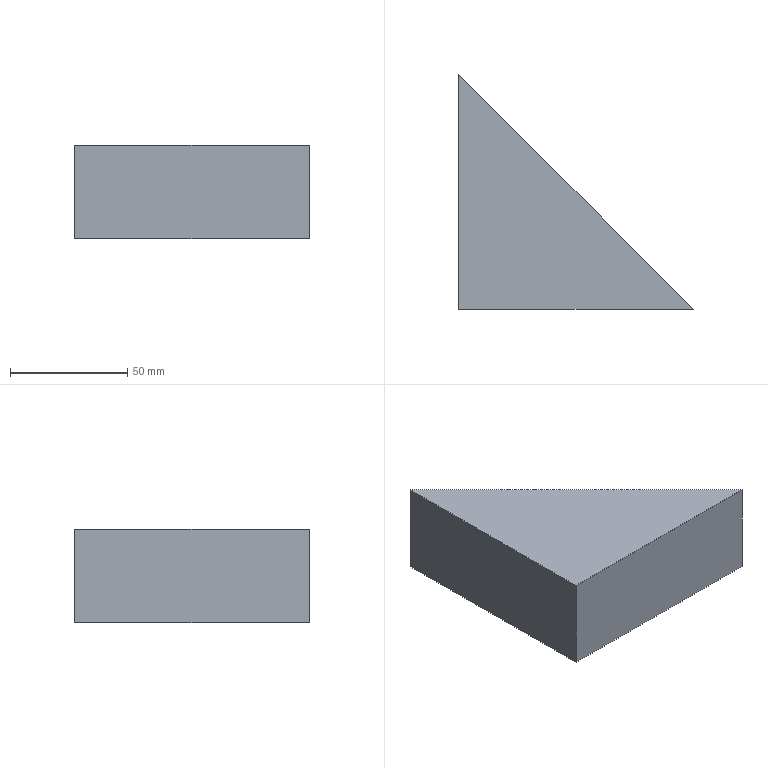Part | 1 solid | 9 faces | box 100 x 100 x 40 mm | volume 67460 mm3 | plane 9
STEP:
#1=CARTESIAN_POINT('',(3.,97.,35.));
#2=VERTEX_POINT('',#1);
#3=CARTESIAN_POINT('',(3.,97.,5.));
#4=VERTEX_POINT('',#3);
#5=CARTESIAN_POINT('',(3.,97.,40.));
#6=DIRECTION('',(0.,0.,-1.));
#7=VECTOR('',#6,1000.);
#8=LINE('',#5,#7);
#9=EDGE_CURVE('',#2,#4,#8,.T.);
#10=ORIENTED_EDGE('',*,*,#9,.T.);
#11=CARTESIAN_POINT('',(97.,3.,5.));
#12=VERTEX_POINT('',#11);
#13=CARTESIAN_POINT('',(100.,0.,5.));
#14=DIRECTION('',(0.7071,-0.7071,0.));
#15=VECTOR('',#14,1000.);
#16=LINE('',#13,#15);
#17=EDGE_CURVE('',#4,#12,#16,.T.);
#18=ORIENTED_EDGE('',*,*,#17,.T.);
#19=CARTESIAN_POINT('',(97.,3.,35.));
#20=VERTEX_POINT('',#19);
#21=CARTESIAN_POINT('',(97.,3.,40.));
#22=DIRECTION('',(0.,0.,1.));
#23=VECTOR('',#22,1000.);
#24=LINE('',#21,#23);
#25=EDGE_CURVE('',#12,#20,#24,.T.);
#26=ORIENTED_EDGE('',*,*,#25,.T.);
#27=CARTESIAN_POINT('',(100.,0.,35.));
#28=DIRECTION('',(0.7071,-0.7071,0.));
#29=VECTOR('',#28,1000.);
#30=LINE('',#27,#29);
#31=EDGE_CURVE('',#2,#20,#30,.T.);
#32=ORIENTED_EDGE('',*,*,#31,.F.);
#33=EDGE_LOOP('',(#10,#18,#26,#32));
#34=FACE_BOUND('',#33,.T.);
#35=CARTESIAN_POINT('',(100.,0.,0.));
#36=VERTEX_POINT('',#35);
#37=CARTESIAN_POINT('',(0.,100.,0.));
#38=VERTEX_POINT('',#37);
#39=CARTESIAN_POINT('',(100.,0.,0.));
#40=DIRECTION('',(-0.7071,0.7071,0.));
#41=VECTOR('',#40,1000.);
#42=LINE('',#39,#41);
#43=EDGE_CURVE('',#36,#38,#42,.T.);
#44=ORIENTED_EDGE('',*,*,#43,.T.);
#45=CARTESIAN_POINT('',(0.,100.,40.));
#46=VERTEX_POINT('',#45);
#47=CARTESIAN_POINT('',(0.,100.,40.));
#48=DIRECTION('',(0.,0.,-1.));
#49=VECTOR('',#48,1000.);
#50=LINE('',#47,#49);
#51=EDGE_CURVE('',#46,#38,#50,.T.);
#52=ORIENTED_EDGE('',*,*,#51,.F.);
#53=CARTESIAN_POINT('',(100.,0.,40.));
#54=VERTEX_POINT('',#53);
#55=CARTESIAN_POINT('',(100.,0.,40.));
#56=DIRECTION('',(-0.7071,0.7071,0.));
#57=VECTOR('',#56,1000.);
#58=LINE('',#55,#57);
#59=EDGE_CURVE('',#54,#46,#58,.T.);
#60=ORIENTED_EDGE('',*,*,#59,.F.);
#61=CARTESIAN_POINT('',(100.,0.,40.));
#62=DIRECTION('',(0.,0.,-1.));
#63=VECTOR('',#62,1000.);
#64=LINE('',#61,#63);
#65=EDGE_CURVE('',#54,#36,#64,.T.);
#66=ORIENTED_EDGE('',*,*,#65,.T.);
#67=EDGE_LOOP('',(#44,#52,#60,#66));
#68=FACE_OUTER_BOUND('',#67,.T.);
#69=CARTESIAN_POINT('',(100.,0.,40.));
#70=DIRECTION('',(-0.7071,-0.7071,0.));
#71=DIRECTION('',(0.7071,-0.7071,0.));
#72=AXIS2_PLACEMENT_3D('',#69,#70,#71);
#73=PLANE('',#72);
#74=ADVANCED_FACE('',(#34,#68),#73,.F.);
#75=CARTESIAN_POINT('',(0.,0.,0.));
#76=VERTEX_POINT('',#75);
#77=CARTESIAN_POINT('',(0.,100.,0.));
#78=DIRECTION('',(0.,-1.,0.));
#79=VECTOR('',#78,1000.);
#80=LINE('',#77,#79);
#81=EDGE_CURVE('',#38,#76,#80,.T.);
#82=ORIENTED_EDGE('',*,*,#81,.T.);
#83=CARTESIAN_POINT('',(0.,0.,40.));
#84=VERTEX_POINT('',#83);
#85=CARTESIAN_POINT('',(0.,0.,40.));
#86=DIRECTION('',(0.,0.,-1.));
#87=VECTOR('',#86,1000.);
#88=LINE('',#85,#87);
#89=EDGE_CURVE('',#84,#76,#88,.T.);
#90=ORIENTED_EDGE('',*,*,#89,.F.);
#91=CARTESIAN_POINT('',(0.,100.,40.));
#92=DIRECTION('',(0.,-1.,0.));
#93=VECTOR('',#92,1000.);
#94=LINE('',#91,#93);
#95=EDGE_CURVE('',#46,#84,#94,.T.);
#96=ORIENTED_EDGE('',*,*,#95,.F.);
#97=ORIENTED_EDGE('',*,*,#51,.T.);
#98=EDGE_LOOP('',(#82,#90,#96,#97));
#99=FACE_OUTER_BOUND('',#98,.T.);
#100=CARTESIAN_POINT('',(0.,100.,40.));
#101=DIRECTION('',(1.,0.,0.));
#102=DIRECTION('',(0.,1.,0.));
#103=AXIS2_PLACEMENT_3D('',#100,#101,#102);
#104=PLANE('',#103);
#105=ADVANCED_FACE('',(#99),#104,.F.);
#106=CARTESIAN_POINT('',(0.,0.,0.));
#107=DIRECTION('',(1.,0.,0.));
#108=VECTOR('',#107,1000.);
#109=LINE('',#106,#108);
#110=EDGE_CURVE('',#76,#36,#109,.T.);
#111=ORIENTED_EDGE('',*,*,#110,.T.);
#112=ORIENTED_EDGE('',*,*,#65,.F.);
#113=CARTESIAN_POINT('',(0.,0.,40.));
#114=DIRECTION('',(1.,0.,0.));
#115=VECTOR('',#114,1000.);
#116=LINE('',#113,#115);
#117=EDGE_CURVE('',#84,#54,#116,.T.);
#118=ORIENTED_EDGE('',*,*,#117,.F.);
#119=ORIENTED_EDGE('',*,*,#89,.T.);
#120=EDGE_LOOP('',(#111,#112,#118,#119));
#121=FACE_OUTER_BOUND('',#120,.T.);
#122=CARTESIAN_POINT('',(0.,0.,40.));
#123=DIRECTION('',(0.,1.,0.));
#124=DIRECTION('',(0.,0.,1.));
#125=AXIS2_PLACEMENT_3D('',#122,#123,#124);
#126=PLANE('',#125);
#127=ADVANCED_FACE('',(#121),#126,.F.);
#128=ORIENTED_EDGE('',*,*,#59,.T.);
#129=ORIENTED_EDGE('',*,*,#95,.T.);
#130=ORIENTED_EDGE('',*,*,#117,.T.);
#131=EDGE_LOOP('',(#128,#129,#130));
#132=FACE_OUTER_BOUND('',#131,.T.);
#133=CARTESIAN_POINT('',(0.,0.,40.));
#134=DIRECTION('',(0.,0.,1.));
#135=DIRECTION('',(1.,0.,0.));
#136=AXIS2_PLACEMENT_3D('',#133,#134,#135);
#137=PLANE('',#136);
#138=ADVANCED_FACE('',(#132),#137,.T.);
#139=ORIENTED_EDGE('',*,*,#43,.F.);
#140=ORIENTED_EDGE('',*,*,#110,.F.);
#141=ORIENTED_EDGE('',*,*,#81,.F.);
#142=EDGE_LOOP('',(#139,#140,#141));
#143=FACE_OUTER_BOUND('',#142,.T.);
#144=CARTESIAN_POINT('',(0.,0.,0.));
#145=DIRECTION('',(0.,0.,1.));
#146=DIRECTION('',(1.,0.,0.));
#147=AXIS2_PLACEMENT_3D('',#144,#145,#146);
#148=PLANE('',#147);
#149=ADVANCED_FACE('',(#143),#148,.F.);
#150=CARTESIAN_POINT('',(3.,3.,5.));
#151=VERTEX_POINT('',#150);
#152=CARTESIAN_POINT('',(3.,3.,5.));
#153=DIRECTION('',(1.,0.,0.));
#154=VECTOR('',#153,1000.);
#155=LINE('',#152,#154);
#156=EDGE_CURVE('',#151,#12,#155,.T.);
#157=ORIENTED_EDGE('',*,*,#156,.F.);
#158=CARTESIAN_POINT('',(3.,3.,35.));
#159=VERTEX_POINT('',#158);
#160=CARTESIAN_POINT('',(3.,3.,5.));
#161=DIRECTION('',(0.,0.,1.));
#162=VECTOR('',#161,1000.);
#163=LINE('',#160,#162);
#164=EDGE_CURVE('',#151,#159,#163,.T.);
#165=ORIENTED_EDGE('',*,*,#164,.T.);
#166=CARTESIAN_POINT('',(3.,3.,35.));
#167=DIRECTION('',(1.,0.,0.));
#168=VECTOR('',#167,1000.);
#169=LINE('',#166,#168);
#170=EDGE_CURVE('',#159,#20,#169,.T.);
#171=ORIENTED_EDGE('',*,*,#170,.T.);
#172=ORIENTED_EDGE('',*,*,#25,.F.);
#173=EDGE_LOOP('',(#157,#165,#171,#172));
#174=FACE_OUTER_BOUND('',#173,.T.);
#175=CARTESIAN_POINT('',(3.,3.,5.));
#176=DIRECTION('',(0.,-1.,0.));
#177=DIRECTION('',(0.,0.,-1.));
#178=AXIS2_PLACEMENT_3D('',#175,#176,#177);
#179=PLANE('',#178);
#180=ADVANCED_FACE('',(#174),#179,.F.);
#181=CARTESIAN_POINT('',(3.,101.243,35.));
#182=DIRECTION('',(0.,-1.,0.));
#183=VECTOR('',#182,1000.);
#184=LINE('',#181,#183);
#185=EDGE_CURVE('',#2,#159,#184,.T.);
#186=ORIENTED_EDGE('',*,*,#185,.T.);
#187=ORIENTED_EDGE('',*,*,#164,.F.);
#188=CARTESIAN_POINT('',(3.,101.243,5.));
#189=DIRECTION('',(0.,-1.,0.));
#190=VECTOR('',#189,1000.);
#191=LINE('',#188,#190);
#192=EDGE_CURVE('',#4,#151,#191,.T.);
#193=ORIENTED_EDGE('',*,*,#192,.F.);
#194=ORIENTED_EDGE('',*,*,#9,.F.);
#195=EDGE_LOOP('',(#186,#187,#193,#194));
#196=FACE_OUTER_BOUND('',#195,.T.);
#197=CARTESIAN_POINT('',(3.,101.243,5.));
#198=DIRECTION('',(-1.,0.,0.));
#199=DIRECTION('',(0.,-1.,0.));
#200=AXIS2_PLACEMENT_3D('',#197,#198,#199);
#201=PLANE('',#200);
#202=ADVANCED_FACE('',(#196),#201,.F.);
#203=ORIENTED_EDGE('',*,*,#192,.T.);
#204=ORIENTED_EDGE('',*,*,#156,.T.);
#205=ORIENTED_EDGE('',*,*,#17,.F.);
#206=EDGE_LOOP('',(#203,#204,#205));
#207=FACE_OUTER_BOUND('',#206,.T.);
#208=CARTESIAN_POINT('',(0.,0.,5.));
#209=DIRECTION('',(0.,0.,-1.));
#210=DIRECTION('',(-1.,0.,0.));
#211=AXIS2_PLACEMENT_3D('',#208,#209,#210);
#212=PLANE('',#211);
#213=ADVANCED_FACE('',(#207),#212,.F.);
#214=ORIENTED_EDGE('',*,*,#31,.T.);
#215=ORIENTED_EDGE('',*,*,#170,.F.);
#216=ORIENTED_EDGE('',*,*,#185,.F.);
#217=EDGE_LOOP('',(#214,#215,#216));
#218=FACE_OUTER_BOUND('',#217,.T.);
#219=CARTESIAN_POINT('',(0.,0.,35.));
#220=DIRECTION('',(0.,0.,-1.));
#221=DIRECTION('',(-1.,0.,0.));
#222=AXIS2_PLACEMENT_3D('',#219,#220,#221);
#223=PLANE('',#222);
#224=ADVANCED_FACE('',(#218),#223,.T.);
#225=CLOSED_SHELL('',(#74,#105,#127,#138,#149,#180,#202,#213,#224));
#226=MANIFOLD_SOLID_BREP('',#225);
#227=CARTESIAN_POINT('',(0.,0.,0.));
#228=DIRECTION('',(0.,0.,1.));
#229=DIRECTION('',(1.,0.,0.));
#230=AXIS2_PLACEMENT_3D('',#227,#228,#229);
#231=(LENGTH_UNIT()NAMED_UNIT(*)SI_UNIT(.MILLI.,.METRE.));
#232=UNCERTAINTY_MEASURE_WITH_UNIT(LENGTH_MEASURE(0.00001),#231,'','');
#233=(NAMED_UNIT(*)PLANE_ANGLE_UNIT()SI_UNIT($,.RADIAN.));
#234=(NAMED_UNIT(*)SI_UNIT($,.STERADIAN.)SOLID_ANGLE_UNIT());
#235=(GEOMETRIC_REPRESENTATION_CONTEXT(3)GLOBAL_UNCERTAINTY_ASSIGNED_CONTEXT((#232))GLOBAL_UNIT_ASSIGNED_CONTEXT((#231,#233,#234))REPRESENTATION_CONTEXT('',''));
#236=ADVANCED_BREP_SHAPE_REPRESENTATION('',(#226,#230),#235);